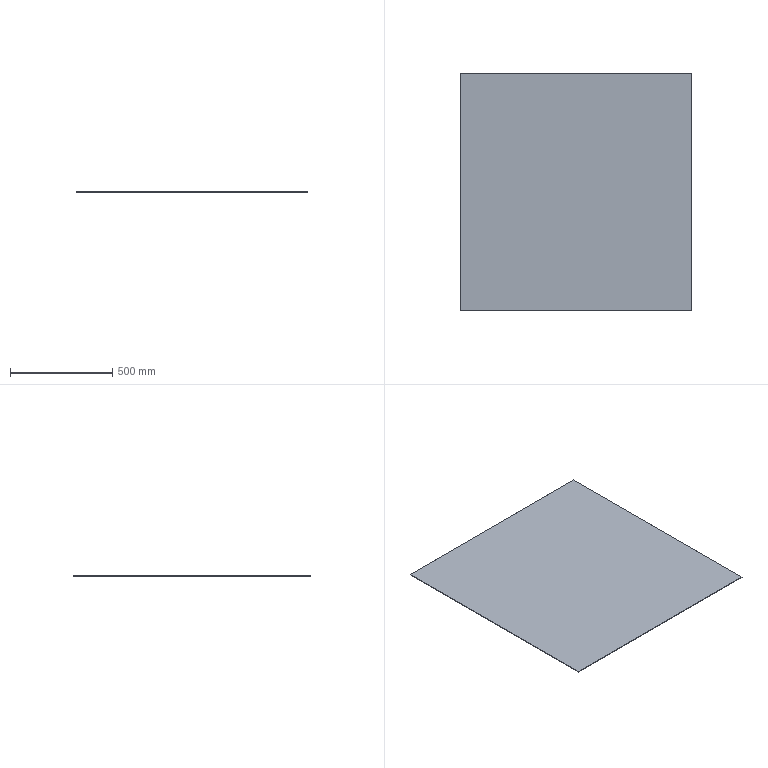Part | 1 solid | 6 faces | box 1135 x 1165 x 3 mm | volume 3966825 mm3 | plane 6
STEP:
#1=CARTESIAN_POINT('',(567.5,-582.5,0.));
#2=VERTEX_POINT('',#1);
#3=CARTESIAN_POINT('',(567.5,582.5,0.));
#4=VERTEX_POINT('',#3);
#5=CARTESIAN_POINT('',(567.5,582.5,0.));
#6=DIRECTION('',(0.,1.,0.));
#7=VECTOR('',#6,1000.);
#8=LINE('',#5,#7);
#9=EDGE_CURVE('',#2,#4,#8,.T.);
#10=ORIENTED_EDGE('',*,*,#9,.T.);
#11=CARTESIAN_POINT('',(567.5,582.5,3.));
#12=VERTEX_POINT('',#11);
#13=CARTESIAN_POINT('',(567.5,582.5,3.));
#14=DIRECTION('',(0.,0.,-1.));
#15=VECTOR('',#14,1000.);
#16=LINE('',#13,#15);
#17=EDGE_CURVE('',#12,#4,#16,.T.);
#18=ORIENTED_EDGE('',*,*,#17,.F.);
#19=CARTESIAN_POINT('',(567.5,-582.5,3.));
#20=VERTEX_POINT('',#19);
#21=CARTESIAN_POINT('',(567.5,582.5,3.));
#22=DIRECTION('',(0.,1.,0.));
#23=VECTOR('',#22,1000.);
#24=LINE('',#21,#23);
#25=EDGE_CURVE('',#20,#12,#24,.T.);
#26=ORIENTED_EDGE('',*,*,#25,.F.);
#27=CARTESIAN_POINT('',(567.5,-582.5,3.));
#28=DIRECTION('',(0.,0.,-1.));
#29=VECTOR('',#28,1000.);
#30=LINE('',#27,#29);
#31=EDGE_CURVE('',#20,#2,#30,.T.);
#32=ORIENTED_EDGE('',*,*,#31,.T.);
#33=EDGE_LOOP('',(#10,#18,#26,#32));
#34=FACE_OUTER_BOUND('',#33,.T.);
#35=CARTESIAN_POINT('',(567.5,582.5,3.));
#36=DIRECTION('',(-1.,0.,0.));
#37=DIRECTION('',(0.,-1.,0.));
#38=AXIS2_PLACEMENT_3D('',#35,#36,#37);
#39=PLANE('',#38);
#40=ADVANCED_FACE('',(#34),#39,.F.);
#41=CARTESIAN_POINT('',(-567.5,582.5,0.));
#42=VERTEX_POINT('',#41);
#43=CARTESIAN_POINT('',(-567.5,582.5,0.));
#44=DIRECTION('',(-1.,0.,0.));
#45=VECTOR('',#44,1000.);
#46=LINE('',#43,#45);
#47=EDGE_CURVE('',#4,#42,#46,.T.);
#48=ORIENTED_EDGE('',*,*,#47,.T.);
#49=CARTESIAN_POINT('',(-567.5,582.5,3.));
#50=VERTEX_POINT('',#49);
#51=CARTESIAN_POINT('',(-567.5,582.5,3.));
#52=DIRECTION('',(0.,0.,-1.));
#53=VECTOR('',#52,1000.);
#54=LINE('',#51,#53);
#55=EDGE_CURVE('',#50,#42,#54,.T.);
#56=ORIENTED_EDGE('',*,*,#55,.F.);
#57=CARTESIAN_POINT('',(-567.5,582.5,3.));
#58=DIRECTION('',(-1.,0.,0.));
#59=VECTOR('',#58,1000.);
#60=LINE('',#57,#59);
#61=EDGE_CURVE('',#12,#50,#60,.T.);
#62=ORIENTED_EDGE('',*,*,#61,.F.);
#63=ORIENTED_EDGE('',*,*,#17,.T.);
#64=EDGE_LOOP('',(#48,#56,#62,#63));
#65=FACE_OUTER_BOUND('',#64,.T.);
#66=CARTESIAN_POINT('',(-567.5,582.5,3.));
#67=DIRECTION('',(0.,-1.,0.));
#68=DIRECTION('',(0.,0.,-1.));
#69=AXIS2_PLACEMENT_3D('',#66,#67,#68);
#70=PLANE('',#69);
#71=ADVANCED_FACE('',(#65),#70,.F.);
#72=CARTESIAN_POINT('',(-567.5,-582.5,0.));
#73=VERTEX_POINT('',#72);
#74=CARTESIAN_POINT('',(-567.5,582.5,0.));
#75=DIRECTION('',(0.,-1.,0.));
#76=VECTOR('',#75,1000.);
#77=LINE('',#74,#76);
#78=EDGE_CURVE('',#42,#73,#77,.T.);
#79=ORIENTED_EDGE('',*,*,#78,.T.);
#80=CARTESIAN_POINT('',(-567.5,-582.5,3.));
#81=VERTEX_POINT('',#80);
#82=CARTESIAN_POINT('',(-567.5,-582.5,3.));
#83=DIRECTION('',(0.,0.,-1.));
#84=VECTOR('',#83,1000.);
#85=LINE('',#82,#84);
#86=EDGE_CURVE('',#81,#73,#85,.T.);
#87=ORIENTED_EDGE('',*,*,#86,.F.);
#88=CARTESIAN_POINT('',(-567.5,582.5,3.));
#89=DIRECTION('',(0.,-1.,0.));
#90=VECTOR('',#89,1000.);
#91=LINE('',#88,#90);
#92=EDGE_CURVE('',#50,#81,#91,.T.);
#93=ORIENTED_EDGE('',*,*,#92,.F.);
#94=ORIENTED_EDGE('',*,*,#55,.T.);
#95=EDGE_LOOP('',(#79,#87,#93,#94));
#96=FACE_OUTER_BOUND('',#95,.T.);
#97=CARTESIAN_POINT('',(-567.5,582.5,3.));
#98=DIRECTION('',(1.,0.,0.));
#99=DIRECTION('',(0.,1.,0.));
#100=AXIS2_PLACEMENT_3D('',#97,#98,#99);
#101=PLANE('',#100);
#102=ADVANCED_FACE('',(#96),#101,.F.);
#103=CARTESIAN_POINT('',(-567.5,-582.5,0.));
#104=DIRECTION('',(1.,0.,0.));
#105=VECTOR('',#104,1000.);
#106=LINE('',#103,#105);
#107=EDGE_CURVE('',#73,#2,#106,.T.);
#108=ORIENTED_EDGE('',*,*,#107,.T.);
#109=ORIENTED_EDGE('',*,*,#31,.F.);
#110=CARTESIAN_POINT('',(-567.5,-582.5,3.));
#111=DIRECTION('',(1.,0.,0.));
#112=VECTOR('',#111,1000.);
#113=LINE('',#110,#112);
#114=EDGE_CURVE('',#81,#20,#113,.T.);
#115=ORIENTED_EDGE('',*,*,#114,.F.);
#116=ORIENTED_EDGE('',*,*,#86,.T.);
#117=EDGE_LOOP('',(#108,#109,#115,#116));
#118=FACE_OUTER_BOUND('',#117,.T.);
#119=CARTESIAN_POINT('',(-567.5,-582.5,3.));
#120=DIRECTION('',(0.,1.,0.));
#121=DIRECTION('',(0.,0.,1.));
#122=AXIS2_PLACEMENT_3D('',#119,#120,#121);
#123=PLANE('',#122);
#124=ADVANCED_FACE('',(#118),#123,.F.);
#125=ORIENTED_EDGE('',*,*,#25,.T.);
#126=ORIENTED_EDGE('',*,*,#61,.T.);
#127=ORIENTED_EDGE('',*,*,#92,.T.);
#128=ORIENTED_EDGE('',*,*,#114,.T.);
#129=EDGE_LOOP('',(#125,#126,#127,#128));
#130=FACE_OUTER_BOUND('',#129,.T.);
#131=CARTESIAN_POINT('',(0.,0.,3.));
#132=DIRECTION('',(0.,0.,1.));
#133=DIRECTION('',(1.,0.,0.));
#134=AXIS2_PLACEMENT_3D('',#131,#132,#133);
#135=PLANE('',#134);
#136=ADVANCED_FACE('',(#130),#135,.T.);
#137=ORIENTED_EDGE('',*,*,#9,.F.);
#138=ORIENTED_EDGE('',*,*,#107,.F.);
#139=ORIENTED_EDGE('',*,*,#78,.F.);
#140=ORIENTED_EDGE('',*,*,#47,.F.);
#141=EDGE_LOOP('',(#137,#138,#139,#140));
#142=FACE_OUTER_BOUND('',#141,.T.);
#143=CARTESIAN_POINT('',(0.,0.,0.));
#144=DIRECTION('',(0.,0.,1.));
#145=DIRECTION('',(1.,0.,0.));
#146=AXIS2_PLACEMENT_3D('',#143,#144,#145);
#147=PLANE('',#146);
#148=ADVANCED_FACE('',(#142),#147,.F.);
#149=CLOSED_SHELL('',(#40,#71,#102,#124,#136,#148));
#150=MANIFOLD_SOLID_BREP('',#149);
#151=CARTESIAN_POINT('',(0.,0.,0.));
#152=DIRECTION('',(0.,0.,1.));
#153=DIRECTION('',(1.,0.,0.));
#154=AXIS2_PLACEMENT_3D('',#151,#152,#153);
#155=(LENGTH_UNIT()NAMED_UNIT(*)SI_UNIT(.MILLI.,.METRE.));
#156=UNCERTAINTY_MEASURE_WITH_UNIT(LENGTH_MEASURE(0.00001),#155,'','');
#157=(NAMED_UNIT(*)PLANE_ANGLE_UNIT()SI_UNIT($,.RADIAN.));
#158=(NAMED_UNIT(*)SI_UNIT($,.STERADIAN.)SOLID_ANGLE_UNIT());
#159=(GEOMETRIC_REPRESENTATION_CONTEXT(3)GLOBAL_UNCERTAINTY_ASSIGNED_CONTEXT((#156))GLOBAL_UNIT_ASSIGNED_CONTEXT((#155,#157,#158))REPRESENTATION_CONTEXT('',''));
#160=ADVANCED_BREP_SHAPE_REPRESENTATION('',(#150,#154),#159);